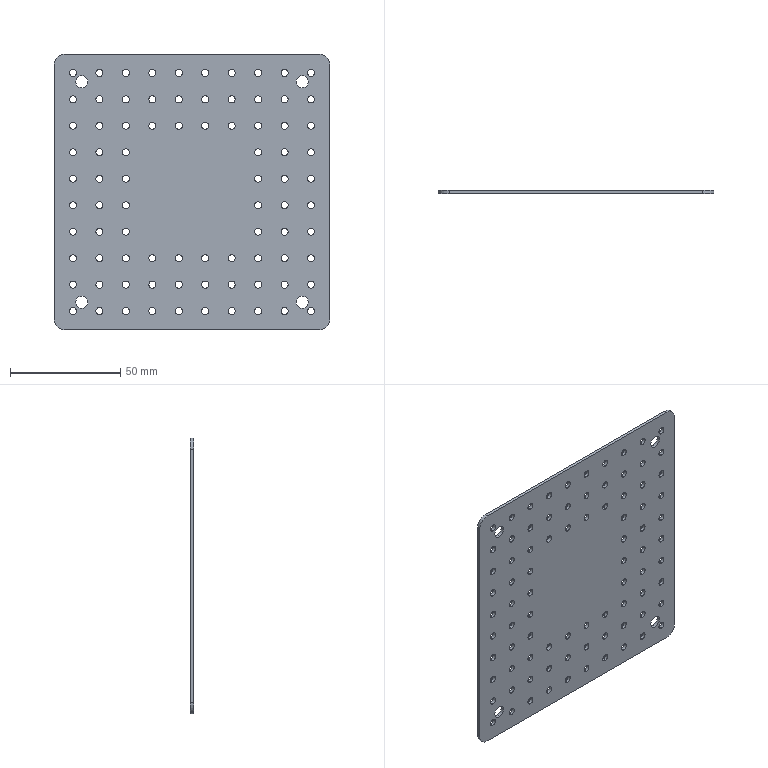Part | SolidWorks | features ICE 3, BaseBody 1 | 1 solid | 186 faces | box 125 x 1.5 x 125 mm | volume 22249 mm3 | cylinder 180 | plane 6 | commonest cylinder face diameters 3.2 x168 5.5 x8 10 x4